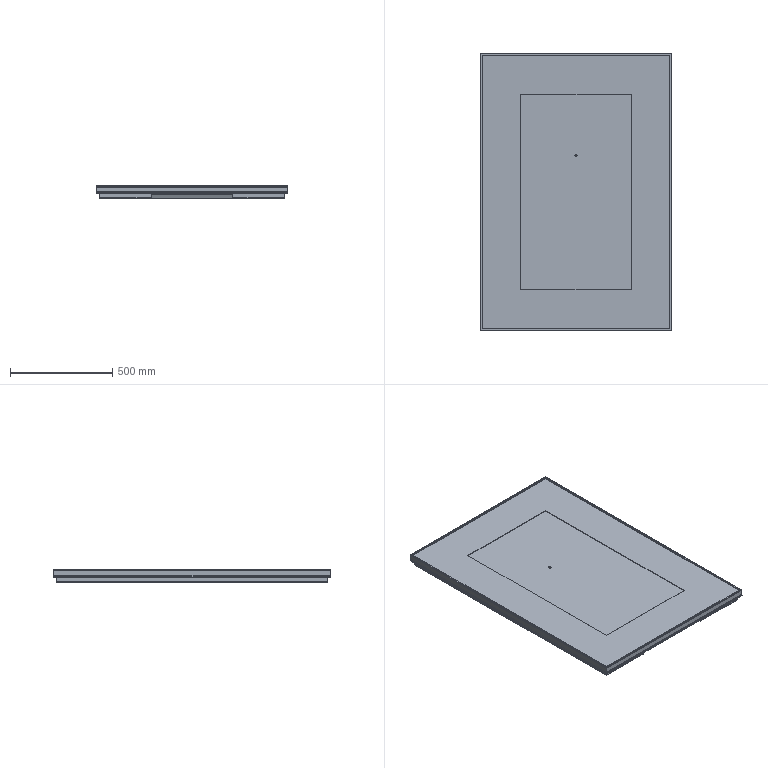Part | SolidWorks | 7 solids | 268 faces | box 940 x 1360 x 60.087 mm | volume 4245748 mm3 | plane 180 | cylinder 76 | spline 12 | commonest cylinder face diameters 7 x30 11 x16 0.4 x9 2.4 x9 2 x6 1 x4